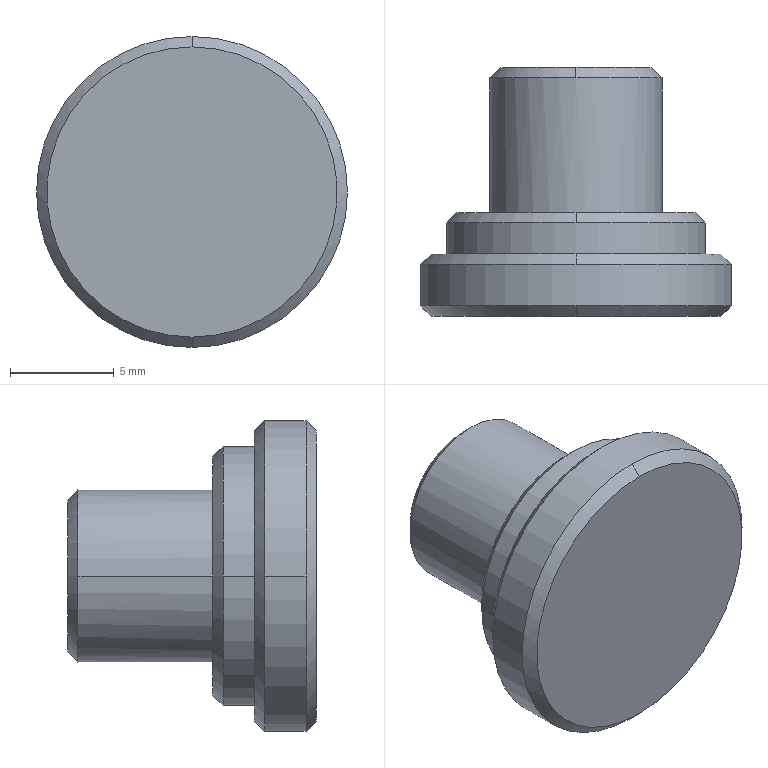Part | SolidWorks | features Chamfer 1, Revolution 1 | 1 solid | 18 faces | box 15 x 12 x 15 mm | volume 1135 mm3 | cone 8 | cylinder 6 | plane 4 | commonest cylinder face diameters 8.3 x2 12.5 x2 15 x2
STEP:
#1=CARTESIAN_POINT('',(148.628,-562.505,3.65));
#2=VERTEX_POINT('',#1);
#3=CARTESIAN_POINT('',(148.628,-562.505,-3.65));
#4=VERTEX_POINT('',#3);
#5=CARTESIAN_POINT('',(148.628,-562.505,0.));
#6=DIRECTION('',(0.,1.,0.));
#7=DIRECTION('',(1.,0.,0.));
#8=AXIS2_PLACEMENT_3D('',#5,#6,#7);
#9=CIRCLE('',#8,3.65);
#10=EDGE_CURVE('',#2,#4,#9,.T.);
#11=ORIENTED_EDGE('',*,*,#10,.F.);
#12=CARTESIAN_POINT('',(148.628,-563.005,4.15));
#13=VERTEX_POINT('',#12);
#14=CARTESIAN_POINT('',(148.628,-562.505,3.65));
#15=DIRECTION('',(0.,-0.7071,0.7071));
#16=VECTOR('',#15,1000.);
#17=LINE('',#14,#16);
#18=EDGE_CURVE('',#2,#13,#17,.T.);
#19=ORIENTED_EDGE('',*,*,#18,.T.);
#20=CARTESIAN_POINT('',(152.778,-563.005,0.));
#21=VERTEX_POINT('',#20);
#22=CARTESIAN_POINT('',(148.628,-563.005,0.));
#23=DIRECTION('',(0.,-1.,0.));
#24=DIRECTION('',(0.,0.,-1.));
#25=AXIS2_PLACEMENT_3D('',#22,#23,#24);
#26=CIRCLE('',#25,4.15);
#27=EDGE_CURVE('',#21,#13,#26,.T.);
#28=ORIENTED_EDGE('',*,*,#27,.F.);
#29=CARTESIAN_POINT('',(148.628,-563.005,-4.15));
#30=VERTEX_POINT('',#29);
#31=CARTESIAN_POINT('',(148.628,-563.005,0.));
#32=DIRECTION('',(0.,-1.,0.));
#33=DIRECTION('',(0.,0.,-1.));
#34=AXIS2_PLACEMENT_3D('',#31,#32,#33);
#35=CIRCLE('',#34,4.15);
#36=EDGE_CURVE('',#30,#21,#35,.T.);
#37=ORIENTED_EDGE('',*,*,#36,.F.);
#38=CARTESIAN_POINT('',(148.628,-562.505,-3.65));
#39=DIRECTION('',(0.,-0.7071,-0.7071));
#40=VECTOR('',#39,1000.);
#41=LINE('',#38,#40);
#42=EDGE_CURVE('',#4,#30,#41,.T.);
#43=ORIENTED_EDGE('',*,*,#42,.F.);
#44=EDGE_LOOP('',(#11,#19,#28,#37,#43));
#45=FACE_OUTER_BOUND('',#44,.T.);
#46=CARTESIAN_POINT('',(148.628,-562.505,0.));
#47=DIRECTION('',(0.,-1.,0.));
#48=DIRECTION('',(0.,0.,-1.));
#49=AXIS2_PLACEMENT_3D('',#46,#47,#48);
#50=CONICAL_SURFACE('',#49,3.65,0.7854);
#51=ADVANCED_FACE('',(#45),#50,.T.);
#52=CARTESIAN_POINT('',(148.628,-569.505,5.75));
#53=VERTEX_POINT('',#52);
#54=CARTESIAN_POINT('',(148.628,-569.505,-5.75));
#55=VERTEX_POINT('',#54);
#56=CARTESIAN_POINT('',(148.628,-569.505,0.));
#57=DIRECTION('',(0.,1.,0.));
#58=DIRECTION('',(1.,0.,0.));
#59=AXIS2_PLACEMENT_3D('',#56,#57,#58);
#60=CIRCLE('',#59,5.75);
#61=EDGE_CURVE('',#53,#55,#60,.T.);
#62=ORIENTED_EDGE('',*,*,#61,.F.);
#63=CARTESIAN_POINT('',(148.628,-570.005,6.25));
#64=VERTEX_POINT('',#63);
#65=CARTESIAN_POINT('',(148.628,-569.505,5.75));
#66=DIRECTION('',(0.,-0.7071,0.7071));
#67=VECTOR('',#66,1000.);
#68=LINE('',#65,#67);
#69=EDGE_CURVE('',#53,#64,#68,.T.);
#70=ORIENTED_EDGE('',*,*,#69,.T.);
#71=CARTESIAN_POINT('',(154.878,-570.005,0.));
#72=VERTEX_POINT('',#71);
#73=CARTESIAN_POINT('',(148.628,-570.005,0.));
#74=DIRECTION('',(0.,-1.,0.));
#75=DIRECTION('',(0.,0.,-1.));
#76=AXIS2_PLACEMENT_3D('',#73,#74,#75);
#77=CIRCLE('',#76,6.25);
#78=EDGE_CURVE('',#72,#64,#77,.T.);
#79=ORIENTED_EDGE('',*,*,#78,.F.);
#80=CARTESIAN_POINT('',(148.628,-570.005,-6.25));
#81=VERTEX_POINT('',#80);
#82=CARTESIAN_POINT('',(148.628,-570.005,0.));
#83=DIRECTION('',(0.,-1.,0.));
#84=DIRECTION('',(0.,0.,-1.));
#85=AXIS2_PLACEMENT_3D('',#82,#83,#84);
#86=CIRCLE('',#85,6.25);
#87=EDGE_CURVE('',#81,#72,#86,.T.);
#88=ORIENTED_EDGE('',*,*,#87,.F.);
#89=CARTESIAN_POINT('',(148.628,-569.505,-5.75));
#90=DIRECTION('',(0.,-0.7071,-0.7071));
#91=VECTOR('',#90,1000.);
#92=LINE('',#89,#91);
#93=EDGE_CURVE('',#55,#81,#92,.T.);
#94=ORIENTED_EDGE('',*,*,#93,.F.);
#95=EDGE_LOOP('',(#62,#70,#79,#88,#94));
#96=FACE_OUTER_BOUND('',#95,.T.);
#97=CARTESIAN_POINT('',(148.628,-569.505,0.));
#98=DIRECTION('',(0.,-1.,0.));
#99=DIRECTION('',(0.,0.,-1.));
#100=AXIS2_PLACEMENT_3D('',#97,#98,#99);
#101=CONICAL_SURFACE('',#100,5.75,0.7854);
#102=ADVANCED_FACE('',(#96),#101,.T.);
#103=CARTESIAN_POINT('',(148.628,-571.505,7.));
#104=VERTEX_POINT('',#103);
#105=CARTESIAN_POINT('',(148.628,-571.505,-7.));
#106=VERTEX_POINT('',#105);
#107=CARTESIAN_POINT('',(148.628,-571.505,0.));
#108=DIRECTION('',(0.,1.,0.));
#109=DIRECTION('',(1.,0.,0.));
#110=AXIS2_PLACEMENT_3D('',#107,#108,#109);
#111=CIRCLE('',#110,7.);
#112=EDGE_CURVE('',#104,#106,#111,.T.);
#113=ORIENTED_EDGE('',*,*,#112,.F.);
#114=CARTESIAN_POINT('',(148.628,-572.005,7.5));
#115=VERTEX_POINT('',#114);
#116=CARTESIAN_POINT('',(148.628,-571.505,7.));
#117=DIRECTION('',(0.,-0.7071,0.7071));
#118=VECTOR('',#117,1000.);
#119=LINE('',#116,#118);
#120=EDGE_CURVE('',#104,#115,#119,.T.);
#121=ORIENTED_EDGE('',*,*,#120,.T.);
#122=CARTESIAN_POINT('',(156.128,-572.005,0.));
#123=VERTEX_POINT('',#122);
#124=CARTESIAN_POINT('',(148.628,-572.005,0.));
#125=DIRECTION('',(0.,-1.,0.));
#126=DIRECTION('',(0.,0.,-1.));
#127=AXIS2_PLACEMENT_3D('',#124,#125,#126);
#128=CIRCLE('',#127,7.5);
#129=EDGE_CURVE('',#123,#115,#128,.T.);
#130=ORIENTED_EDGE('',*,*,#129,.F.);
#131=CARTESIAN_POINT('',(148.628,-572.005,-7.5));
#132=VERTEX_POINT('',#131);
#133=CARTESIAN_POINT('',(148.628,-572.005,0.));
#134=DIRECTION('',(0.,-1.,0.));
#135=DIRECTION('',(0.,0.,-1.));
#136=AXIS2_PLACEMENT_3D('',#133,#134,#135);
#137=CIRCLE('',#136,7.5);
#138=EDGE_CURVE('',#132,#123,#137,.T.);
#139=ORIENTED_EDGE('',*,*,#138,.F.);
#140=CARTESIAN_POINT('',(148.628,-571.505,-7.));
#141=DIRECTION('',(0.,-0.7071,-0.7071));
#142=VECTOR('',#141,1000.);
#143=LINE('',#140,#142);
#144=EDGE_CURVE('',#106,#132,#143,.T.);
#145=ORIENTED_EDGE('',*,*,#144,.F.);
#146=EDGE_LOOP('',(#113,#121,#130,#139,#145));
#147=FACE_OUTER_BOUND('',#146,.T.);
#148=CARTESIAN_POINT('',(148.628,-571.505,0.));
#149=DIRECTION('',(0.,-1.,0.));
#150=DIRECTION('',(0.,0.,-1.));
#151=AXIS2_PLACEMENT_3D('',#148,#149,#150);
#152=CONICAL_SURFACE('',#151,7.,0.7854);
#153=ADVANCED_FACE('',(#147),#152,.T.);
#154=CARTESIAN_POINT('',(148.628,-574.505,-7.));
#155=VERTEX_POINT('',#154);
#156=CARTESIAN_POINT('',(148.628,-574.505,7.));
#157=VERTEX_POINT('',#156);
#158=CARTESIAN_POINT('',(148.628,-574.505,0.));
#159=DIRECTION('',(0.,-1.,0.));
#160=DIRECTION('',(-1.,0.,0.));
#161=AXIS2_PLACEMENT_3D('',#158,#159,#160);
#162=CIRCLE('',#161,7.);
#163=EDGE_CURVE('',#155,#157,#162,.T.);
#164=ORIENTED_EDGE('',*,*,#163,.F.);
#165=CARTESIAN_POINT('',(148.628,-574.005,-7.5));
#166=VERTEX_POINT('',#165);
#167=CARTESIAN_POINT('',(148.628,-574.005,-7.5));
#168=DIRECTION('',(0.,0.7071,-0.7071));
#169=VECTOR('',#168,1000.);
#170=LINE('',#167,#169);
#171=EDGE_CURVE('',#155,#166,#170,.T.);
#172=ORIENTED_EDGE('',*,*,#171,.T.);
#173=CARTESIAN_POINT('',(156.128,-574.005,0.));
#174=VERTEX_POINT('',#173);
#175=CARTESIAN_POINT('',(148.628,-574.005,0.));
#176=DIRECTION('',(0.,1.,0.));
#177=DIRECTION('',(0.,0.,1.));
#178=AXIS2_PLACEMENT_3D('',#175,#176,#177);
#179=CIRCLE('',#178,7.5);
#180=EDGE_CURVE('',#174,#166,#179,.T.);
#181=ORIENTED_EDGE('',*,*,#180,.F.);
#182=CARTESIAN_POINT('',(148.628,-574.005,7.5));
#183=VERTEX_POINT('',#182);
#184=CARTESIAN_POINT('',(148.628,-574.005,0.));
#185=DIRECTION('',(0.,1.,0.));
#186=DIRECTION('',(0.,0.,1.));
#187=AXIS2_PLACEMENT_3D('',#184,#185,#186);
#188=CIRCLE('',#187,7.5);
#189=EDGE_CURVE('',#183,#174,#188,.T.);
#190=ORIENTED_EDGE('',*,*,#189,.F.);
#191=CARTESIAN_POINT('',(148.628,-574.005,7.5));
#192=DIRECTION('',(0.,0.7071,0.7071));
#193=VECTOR('',#192,1000.);
#194=LINE('',#191,#193);
#195=EDGE_CURVE('',#157,#183,#194,.T.);
#196=ORIENTED_EDGE('',*,*,#195,.F.);
#197=EDGE_LOOP('',(#164,#172,#181,#190,#196));
#198=FACE_OUTER_BOUND('',#197,.T.);
#199=CARTESIAN_POINT('',(148.628,-574.005,0.));
#200=DIRECTION('',(0.,1.,0.));
#201=DIRECTION('',(0.,0.,1.));
#202=AXIS2_PLACEMENT_3D('',#199,#200,#201);
#203=CONICAL_SURFACE('',#202,7.5,0.7854);
#204=ADVANCED_FACE('',(#198),#203,.T.);
#205=CARTESIAN_POINT('',(141.128,-574.005,0.));
#206=VERTEX_POINT('',#205);
#207=CARTESIAN_POINT('',(148.628,-574.005,0.));
#208=DIRECTION('',(0.,1.,0.));
#209=DIRECTION('',(0.,0.,1.));
#210=AXIS2_PLACEMENT_3D('',#207,#208,#209);
#211=CIRCLE('',#210,7.5);
#212=EDGE_CURVE('',#206,#183,#211,.T.);
#213=ORIENTED_EDGE('',*,*,#212,.T.);
#214=ORIENTED_EDGE('',*,*,#189,.T.);
#215=CARTESIAN_POINT('',(156.128,-560.805,0.));
#216=DIRECTION('',(0.,1.,0.));
#217=VECTOR('',#216,1000.);
#218=LINE('',#215,#217);
#219=EDGE_CURVE('',#174,#123,#218,.T.);
#220=ORIENTED_EDGE('',*,*,#219,.T.);
#221=ORIENTED_EDGE('',*,*,#129,.T.);
#222=CARTESIAN_POINT('',(141.128,-572.005,0.));
#223=VERTEX_POINT('',#222);
#224=CARTESIAN_POINT('',(148.628,-572.005,0.));
#225=DIRECTION('',(0.,-1.,0.));
#226=DIRECTION('',(0.,0.,-1.));
#227=AXIS2_PLACEMENT_3D('',#224,#225,#226);
#228=CIRCLE('',#227,7.5);
#229=EDGE_CURVE('',#115,#223,#228,.T.);
#230=ORIENTED_EDGE('',*,*,#229,.T.);
#231=CARTESIAN_POINT('',(141.128,-560.805,0.));
#232=DIRECTION('',(0.,1.,0.));
#233=VECTOR('',#232,1000.);
#234=LINE('',#231,#233);
#235=EDGE_CURVE('',#206,#223,#234,.T.);
#236=ORIENTED_EDGE('',*,*,#235,.F.);
#237=EDGE_LOOP('',(#213,#214,#220,#221,#230,#236));
#238=FACE_OUTER_BOUND('',#237,.T.);
#239=CARTESIAN_POINT('',(148.628,-560.805,0.));
#240=DIRECTION('',(0.,1.,0.));
#241=DIRECTION('',(-1.,0.,0.));
#242=AXIS2_PLACEMENT_3D('',#239,#240,#241);
#243=CYLINDRICAL_SURFACE('',#242,7.5);
#244=ADVANCED_FACE('',(#238),#243,.T.);
#245=CARTESIAN_POINT('',(144.478,-569.505,0.));
#246=VERTEX_POINT('',#245);
#247=CARTESIAN_POINT('',(152.778,-569.505,0.));
#248=VERTEX_POINT('',#247);
#249=CARTESIAN_POINT('',(148.628,-569.505,0.));
#250=DIRECTION('',(0.,1.,0.));
#251=DIRECTION('',(-1.,0.,0.));
#252=AXIS2_PLACEMENT_3D('',#249,#250,#251);
#253=CIRCLE('',#252,4.15);
#254=EDGE_CURVE('',#246,#248,#253,.T.);
#255=ORIENTED_EDGE('',*,*,#254,.T.);
#256=CARTESIAN_POINT('',(152.778,-560.805,0.));
#257=DIRECTION('',(0.,1.,0.));
#258=VECTOR('',#257,1000.);
#259=LINE('',#256,#258);
#260=EDGE_CURVE('',#248,#21,#259,.T.);
#261=ORIENTED_EDGE('',*,*,#260,.T.);
#262=ORIENTED_EDGE('',*,*,#27,.T.);
#263=CARTESIAN_POINT('',(144.478,-563.005,0.));
#264=VERTEX_POINT('',#263);
#265=CARTESIAN_POINT('',(148.628,-563.005,0.));
#266=DIRECTION('',(0.,-1.,0.));
#267=DIRECTION('',(0.,0.,-1.));
#268=AXIS2_PLACEMENT_3D('',#265,#266,#267);
#269=CIRCLE('',#268,4.15);
#270=EDGE_CURVE('',#13,#264,#269,.T.);
#271=ORIENTED_EDGE('',*,*,#270,.T.);
#272=CARTESIAN_POINT('',(144.478,-560.805,0.));
#273=DIRECTION('',(0.,1.,0.));
#274=VECTOR('',#273,1000.);
#275=LINE('',#272,#274);
#276=EDGE_CURVE('',#246,#264,#275,.T.);
#277=ORIENTED_EDGE('',*,*,#276,.F.);
#278=EDGE_LOOP('',(#255,#261,#262,#271,#277));
#279=FACE_OUTER_BOUND('',#278,.T.);
#280=CARTESIAN_POINT('',(148.628,-560.805,0.));
#281=DIRECTION('',(0.,1.,0.));
#282=DIRECTION('',(-1.,0.,0.));
#283=AXIS2_PLACEMENT_3D('',#280,#281,#282);
#284=CYLINDRICAL_SURFACE('',#283,4.15);
#285=ADVANCED_FACE('',(#279),#284,.T.);
#286=CARTESIAN_POINT('',(142.378,-571.505,0.));
#287=VERTEX_POINT('',#286);
#288=CARTESIAN_POINT('',(154.878,-571.505,0.));
#289=VERTEX_POINT('',#288);
#290=CARTESIAN_POINT('',(148.628,-571.505,0.));
#291=DIRECTION('',(0.,1.,0.));
#292=DIRECTION('',(-1.,0.,0.));
#293=AXIS2_PLACEMENT_3D('',#290,#291,#292);
#294=CIRCLE('',#293,6.25);
#295=EDGE_CURVE('',#287,#289,#294,.T.);
#296=ORIENTED_EDGE('',*,*,#295,.T.);
#297=CARTESIAN_POINT('',(154.878,-560.805,0.));
#298=DIRECTION('',(0.,1.,0.));
#299=VECTOR('',#298,1000.);
#300=LINE('',#297,#299);
#301=EDGE_CURVE('',#289,#72,#300,.T.);
#302=ORIENTED_EDGE('',*,*,#301,.T.);
#303=ORIENTED_EDGE('',*,*,#78,.T.);
#304=CARTESIAN_POINT('',(142.378,-570.005,0.));
#305=VERTEX_POINT('',#304);
#306=CARTESIAN_POINT('',(148.628,-570.005,0.));
#307=DIRECTION('',(0.,-1.,0.));
#308=DIRECTION('',(0.,0.,-1.));
#309=AXIS2_PLACEMENT_3D('',#306,#307,#308);
#310=CIRCLE('',#309,6.25);
#311=EDGE_CURVE('',#64,#305,#310,.T.);
#312=ORIENTED_EDGE('',*,*,#311,.T.);
#313=CARTESIAN_POINT('',(142.378,-560.805,0.));
#314=DIRECTION('',(0.,1.,0.));
#315=VECTOR('',#314,1000.);
#316=LINE('',#313,#315);
#317=EDGE_CURVE('',#287,#305,#316,.T.);
#318=ORIENTED_EDGE('',*,*,#317,.F.);
#319=EDGE_LOOP('',(#296,#302,#303,#312,#318));
#320=FACE_OUTER_BOUND('',#319,.T.);
#321=CARTESIAN_POINT('',(148.628,-560.805,0.));
#322=DIRECTION('',(0.,1.,0.));
#323=DIRECTION('',(-1.,0.,0.));
#324=AXIS2_PLACEMENT_3D('',#321,#322,#323);
#325=CYLINDRICAL_SURFACE('',#324,6.25);
#326=ADVANCED_FACE('',(#320),#325,.T.);
#327=ORIENTED_EDGE('',*,*,#301,.F.);
#328=CARTESIAN_POINT('',(148.628,-571.505,0.));
#329=DIRECTION('',(0.,1.,0.));
#330=DIRECTION('',(-1.,0.,0.));
#331=AXIS2_PLACEMENT_3D('',#328,#329,#330);
#332=CIRCLE('',#331,6.25);
#333=EDGE_CURVE('',#289,#287,#332,.T.);
#334=ORIENTED_EDGE('',*,*,#333,.T.);
#335=ORIENTED_EDGE('',*,*,#317,.T.);
#336=CARTESIAN_POINT('',(148.628,-570.005,0.));
#337=DIRECTION('',(0.,-1.,0.));
#338=DIRECTION('',(0.,0.,-1.));
#339=AXIS2_PLACEMENT_3D('',#336,#337,#338);
#340=CIRCLE('',#339,6.25);
#341=EDGE_CURVE('',#305,#81,#340,.T.);
#342=ORIENTED_EDGE('',*,*,#341,.T.);
#343=ORIENTED_EDGE('',*,*,#87,.T.);
#344=EDGE_LOOP('',(#327,#334,#335,#342,#343));
#345=FACE_OUTER_BOUND('',#344,.T.);
#346=CARTESIAN_POINT('',(148.628,-560.805,0.));
#347=DIRECTION('',(0.,1.,0.));
#348=DIRECTION('',(-1.,0.,0.));
#349=AXIS2_PLACEMENT_3D('',#346,#347,#348);
#350=CYLINDRICAL_SURFACE('',#349,6.25);
#351=ADVANCED_FACE('',(#345),#350,.T.);
#352=CARTESIAN_POINT('',(148.628,-569.505,0.));
#353=DIRECTION('',(0.,1.,0.));
#354=DIRECTION('',(1.,0.,0.));
#355=AXIS2_PLACEMENT_3D('',#352,#353,#354);
#356=CIRCLE('',#355,5.75);
#357=EDGE_CURVE('',#55,#53,#356,.T.);
#358=ORIENTED_EDGE('',*,*,#357,.T.);
#359=ORIENTED_EDGE('',*,*,#61,.T.);
#360=EDGE_LOOP('',(#358,#359));
#361=FACE_OUTER_BOUND('',#360,.T.);
#362=ORIENTED_EDGE('',*,*,#254,.F.);
#363=CARTESIAN_POINT('',(148.628,-569.505,0.));
#364=DIRECTION('',(0.,1.,0.));
#365=DIRECTION('',(-1.,0.,0.));
#366=AXIS2_PLACEMENT_3D('',#363,#364,#365);
#367=CIRCLE('',#366,4.15);
#368=EDGE_CURVE('',#248,#246,#367,.T.);
#369=ORIENTED_EDGE('',*,*,#368,.F.);
#370=EDGE_LOOP('',(#362,#369));
#371=FACE_BOUND('',#370,.T.);
#372=CARTESIAN_POINT('',(154.878,-569.505,0.));
#373=DIRECTION('',(0.,-1.,0.));
#374=DIRECTION('',(1.,0.,0.));
#375=AXIS2_PLACEMENT_3D('',#372,#373,#374);
#376=PLANE('',#375);
#377=ADVANCED_FACE('',(#361,#371),#376,.F.);
#378=ORIENTED_EDGE('',*,*,#260,.F.);
#379=ORIENTED_EDGE('',*,*,#368,.T.);
#380=ORIENTED_EDGE('',*,*,#276,.T.);
#381=CARTESIAN_POINT('',(148.628,-563.005,0.));
#382=DIRECTION('',(0.,-1.,0.));
#383=DIRECTION('',(0.,0.,-1.));
#384=AXIS2_PLACEMENT_3D('',#381,#382,#383);
#385=CIRCLE('',#384,4.15);
#386=EDGE_CURVE('',#264,#30,#385,.T.);
#387=ORIENTED_EDGE('',*,*,#386,.T.);
#388=ORIENTED_EDGE('',*,*,#36,.T.);
#389=EDGE_LOOP('',(#378,#379,#380,#387,#388));
#390=FACE_OUTER_BOUND('',#389,.T.);
#391=CARTESIAN_POINT('',(148.628,-560.805,0.));
#392=DIRECTION('',(0.,1.,0.));
#393=DIRECTION('',(-1.,0.,0.));
#394=AXIS2_PLACEMENT_3D('',#391,#392,#393);
#395=CYLINDRICAL_SURFACE('',#394,4.15);
#396=ADVANCED_FACE('',(#390),#395,.T.);
#397=CARTESIAN_POINT('',(148.628,-562.505,0.));
#398=DIRECTION('',(0.,1.,0.));
#399=DIRECTION('',(1.,0.,0.));
#400=AXIS2_PLACEMENT_3D('',#397,#398,#399);
#401=CIRCLE('',#400,3.65);
#402=EDGE_CURVE('',#4,#2,#401,.T.);
#403=ORIENTED_EDGE('',*,*,#402,.T.);
#404=ORIENTED_EDGE('',*,*,#10,.T.);
#405=EDGE_LOOP('',(#403,#404));
#406=FACE_OUTER_BOUND('',#405,.T.);
#407=CARTESIAN_POINT('',(152.778,-562.505,0.));
#408=DIRECTION('',(0.,-1.,0.));
#409=DIRECTION('',(1.,0.,0.));
#410=AXIS2_PLACEMENT_3D('',#407,#408,#409);
#411=PLANE('',#410);
#412=ADVANCED_FACE('',(#406),#411,.F.);
#413=CARTESIAN_POINT('',(148.628,-574.505,0.));
#414=DIRECTION('',(0.,-1.,0.));
#415=DIRECTION('',(-1.,0.,0.));
#416=AXIS2_PLACEMENT_3D('',#413,#414,#415);
#417=CIRCLE('',#416,7.);
#418=EDGE_CURVE('',#157,#155,#417,.T.);
#419=ORIENTED_EDGE('',*,*,#418,.T.);
#420=ORIENTED_EDGE('',*,*,#163,.T.);
#421=EDGE_LOOP('',(#419,#420));
#422=FACE_OUTER_BOUND('',#421,.T.);
#423=CARTESIAN_POINT('',(156.128,-574.505,0.));
#424=DIRECTION('',(0.,1.,0.));
#425=DIRECTION('',(-1.,0.,0.));
#426=AXIS2_PLACEMENT_3D('',#423,#424,#425);
#427=PLANE('',#426);
#428=ADVANCED_FACE('',(#422),#427,.F.);
#429=ORIENTED_EDGE('',*,*,#219,.F.);
#430=ORIENTED_EDGE('',*,*,#180,.T.);
#431=CARTESIAN_POINT('',(148.628,-574.005,0.));
#432=DIRECTION('',(0.,1.,0.));
#433=DIRECTION('',(0.,0.,1.));
#434=AXIS2_PLACEMENT_3D('',#431,#432,#433);
#435=CIRCLE('',#434,7.5);
#436=EDGE_CURVE('',#166,#206,#435,.T.);
#437=ORIENTED_EDGE('',*,*,#436,.T.);
#438=ORIENTED_EDGE('',*,*,#235,.T.);
#439=CARTESIAN_POINT('',(148.628,-572.005,0.));
#440=DIRECTION('',(0.,-1.,0.));
#441=DIRECTION('',(0.,0.,-1.));
#442=AXIS2_PLACEMENT_3D('',#439,#440,#441);
#443=CIRCLE('',#442,7.5);
#444=EDGE_CURVE('',#223,#132,#443,.T.);
#445=ORIENTED_EDGE('',*,*,#444,.T.);
#446=ORIENTED_EDGE('',*,*,#138,.T.);
#447=EDGE_LOOP('',(#429,#430,#437,#438,#445,#446));
#448=FACE_OUTER_BOUND('',#447,.T.);
#449=CARTESIAN_POINT('',(148.628,-560.805,0.));
#450=DIRECTION('',(0.,1.,0.));
#451=DIRECTION('',(-1.,0.,0.));
#452=AXIS2_PLACEMENT_3D('',#449,#450,#451);
#453=CYLINDRICAL_SURFACE('',#452,7.5);
#454=ADVANCED_FACE('',(#448),#453,.T.);
#455=CARTESIAN_POINT('',(148.628,-571.505,0.));
#456=DIRECTION('',(0.,1.,0.));
#457=DIRECTION('',(1.,0.,0.));
#458=AXIS2_PLACEMENT_3D('',#455,#456,#457);
#459=CIRCLE('',#458,7.);
#460=EDGE_CURVE('',#106,#104,#459,.T.);
#461=ORIENTED_EDGE('',*,*,#460,.T.);
#462=ORIENTED_EDGE('',*,*,#112,.T.);
#463=EDGE_LOOP('',(#461,#462));
#464=FACE_OUTER_BOUND('',#463,.T.);
#465=ORIENTED_EDGE('',*,*,#295,.F.);
#466=ORIENTED_EDGE('',*,*,#333,.F.);
#467=EDGE_LOOP('',(#465,#466));
#468=FACE_BOUND('',#467,.T.);
#469=CARTESIAN_POINT('',(154.878,-571.505,0.));
#470=DIRECTION('',(0.,-1.,0.));
#471=DIRECTION('',(1.,0.,0.));
#472=AXIS2_PLACEMENT_3D('',#469,#470,#471);
#473=PLANE('',#472);
#474=ADVANCED_FACE('',(#464,#468),#473,.F.);
#475=ORIENTED_EDGE('',*,*,#171,.F.);
#476=ORIENTED_EDGE('',*,*,#418,.F.);
#477=ORIENTED_EDGE('',*,*,#195,.T.);
#478=ORIENTED_EDGE('',*,*,#212,.F.);
#479=ORIENTED_EDGE('',*,*,#436,.F.);
#480=EDGE_LOOP('',(#475,#476,#477,#478,#479));
#481=FACE_OUTER_BOUND('',#480,.T.);
#482=CARTESIAN_POINT('',(148.628,-574.005,0.));
#483=DIRECTION('',(0.,1.,0.));
#484=DIRECTION('',(0.,0.,1.));
#485=AXIS2_PLACEMENT_3D('',#482,#483,#484);
#486=CONICAL_SURFACE('',#485,7.5,0.7854);
#487=ADVANCED_FACE('',(#481),#486,.T.);
#488=ORIENTED_EDGE('',*,*,#120,.F.);
#489=ORIENTED_EDGE('',*,*,#460,.F.);
#490=ORIENTED_EDGE('',*,*,#144,.T.);
#491=ORIENTED_EDGE('',*,*,#444,.F.);
#492=ORIENTED_EDGE('',*,*,#229,.F.);
#493=EDGE_LOOP('',(#488,#489,#490,#491,#492));
#494=FACE_OUTER_BOUND('',#493,.T.);
#495=CARTESIAN_POINT('',(148.628,-571.505,0.));
#496=DIRECTION('',(0.,-1.,0.));
#497=DIRECTION('',(0.,0.,-1.));
#498=AXIS2_PLACEMENT_3D('',#495,#496,#497);
#499=CONICAL_SURFACE('',#498,7.,0.7854);
#500=ADVANCED_FACE('',(#494),#499,.T.);
#501=ORIENTED_EDGE('',*,*,#69,.F.);
#502=ORIENTED_EDGE('',*,*,#357,.F.);
#503=ORIENTED_EDGE('',*,*,#93,.T.);
#504=ORIENTED_EDGE('',*,*,#341,.F.);
#505=ORIENTED_EDGE('',*,*,#311,.F.);
#506=EDGE_LOOP('',(#501,#502,#503,#504,#505));
#507=FACE_OUTER_BOUND('',#506,.T.);
#508=CARTESIAN_POINT('',(148.628,-569.505,0.));
#509=DIRECTION('',(0.,-1.,0.));
#510=DIRECTION('',(0.,0.,-1.));
#511=AXIS2_PLACEMENT_3D('',#508,#509,#510);
#512=CONICAL_SURFACE('',#511,5.75,0.7854);
#513=ADVANCED_FACE('',(#507),#512,.T.);
#514=ORIENTED_EDGE('',*,*,#18,.F.);
#515=ORIENTED_EDGE('',*,*,#402,.F.);
#516=ORIENTED_EDGE('',*,*,#42,.T.);
#517=ORIENTED_EDGE('',*,*,#386,.F.);
#518=ORIENTED_EDGE('',*,*,#270,.F.);
#519=EDGE_LOOP('',(#514,#515,#516,#517,#518));
#520=FACE_OUTER_BOUND('',#519,.T.);
#521=CARTESIAN_POINT('',(148.628,-562.505,0.));
#522=DIRECTION('',(0.,-1.,0.));
#523=DIRECTION('',(0.,0.,-1.));
#524=AXIS2_PLACEMENT_3D('',#521,#522,#523);
#525=CONICAL_SURFACE('',#524,3.65,0.7854);
#526=ADVANCED_FACE('',(#520),#525,.T.);
#527=CLOSED_SHELL('',(#51,#102,#153,#204,#244,#285,#326,#351,#377,#396,#412,#428,#454,#474,#487,#500,#513,#526));
#528=MANIFOLD_SOLID_BREP('',#527);
#529=CARTESIAN_POINT('',(0.,0.,0.));
#530=DIRECTION('',(0.,0.,1.));
#531=DIRECTION('',(1.,0.,0.));
#532=AXIS2_PLACEMENT_3D('',#529,#530,#531);
#533=(LENGTH_UNIT()NAMED_UNIT(*)SI_UNIT(.MILLI.,.METRE.));
#534=UNCERTAINTY_MEASURE_WITH_UNIT(LENGTH_MEASURE(0.00001),#533,'','');
#535=(NAMED_UNIT(*)PLANE_ANGLE_UNIT()SI_UNIT($,.RADIAN.));
#536=(NAMED_UNIT(*)SI_UNIT($,.STERADIAN.)SOLID_ANGLE_UNIT());
#537=(GEOMETRIC_REPRESENTATION_CONTEXT(3)GLOBAL_UNCERTAINTY_ASSIGNED_CONTEXT((#534))GLOBAL_UNIT_ASSIGNED_CONTEXT((#533,#535,#536))REPRESENTATION_CONTEXT('',''));
#538=ADVANCED_BREP_SHAPE_REPRESENTATION('',(#528,#532),#537);